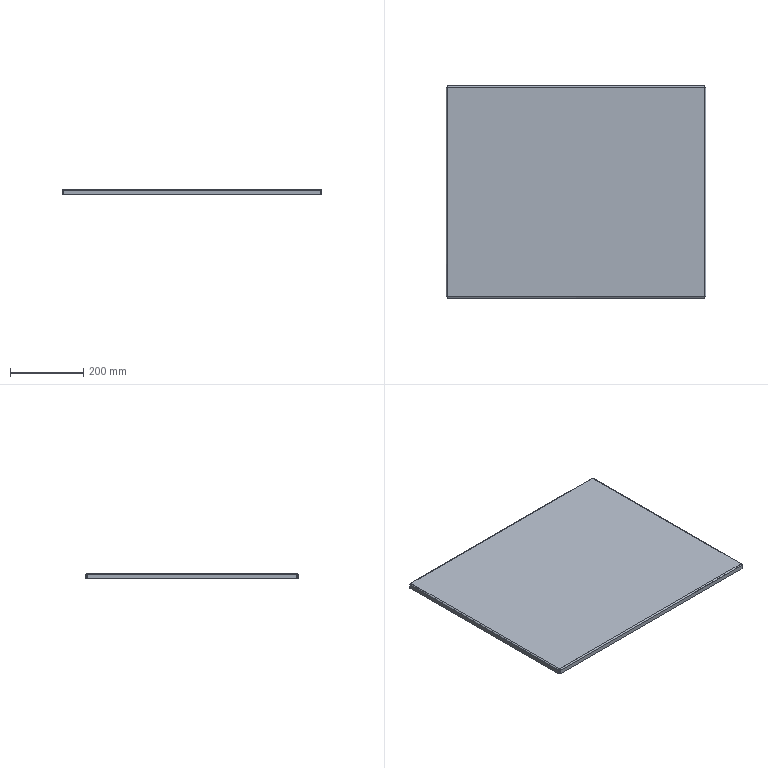Part | STEP file | MYT-A01-P37 | 1 solid | 38 faces | box 710 x 580 x 15 mm | volume 1319701 mm3 | plane 22 | spline 8 | cylinder 8 | commonest cylinder face diameters 1.473 x4 7.473 x4
STEP:
#1=CARTESIAN_POINT('',(-351.263,-286.263,-3.));
#2=VERTEX_POINT('',#1);
#3=CARTESIAN_POINT('',(351.263,-286.263,-3.));
#4=VERTEX_POINT('',#3);
#5=CARTESIAN_POINT('',(-351.293,-286.263,-3.));
#6=DIRECTION('',(1.,0.,0.));
#7=VECTOR('',#6,1000.);
#8=LINE('',#5,#7);
#9=EDGE_CURVE('',#2,#4,#8,.T.);
#10=ORIENTED_EDGE('',*,*,#9,.F.);
#11=CARTESIAN_POINT('',(-351.263,286.263,-3.));
#12=VERTEX_POINT('',#11);
#13=CARTESIAN_POINT('',(-351.263,286.293,-3.));
#14=DIRECTION('',(0.,-1.,0.));
#15=VECTOR('',#14,1000.);
#16=LINE('',#13,#15);
#17=EDGE_CURVE('',#12,#2,#16,.T.);
#18=ORIENTED_EDGE('',*,*,#17,.F.);
#19=CARTESIAN_POINT('',(351.263,286.263,-3.));
#20=VERTEX_POINT('',#19);
#21=CARTESIAN_POINT('',(351.293,286.263,-3.));
#22=DIRECTION('',(-1.,0.,0.));
#23=VECTOR('',#22,1000.);
#24=LINE('',#21,#23);
#25=EDGE_CURVE('',#20,#12,#24,.T.);
#26=ORIENTED_EDGE('',*,*,#25,.F.);
#27=CARTESIAN_POINT('',(351.263,-286.293,-3.));
#28=DIRECTION('',(0.,1.,0.));
#29=VECTOR('',#28,1000.);
#30=LINE('',#27,#29);
#31=EDGE_CURVE('',#4,#20,#30,.T.);
#32=ORIENTED_EDGE('',*,*,#31,.F.);
#33=EDGE_LOOP('',(#10,#18,#26,#32));
#34=FACE_OUTER_BOUND('',#33,.T.);
#35=CARTESIAN_POINT('',(0.,0.,-3.));
#36=DIRECTION('',(0.,0.,1.));
#37=DIRECTION('',(1.,0.,0.));
#38=AXIS2_PLACEMENT_3D('',#35,#36,#37);
#39=PLANE('',#38);
#40=ADVANCED_FACE('',(#34),#39,.F.);
#41=CARTESIAN_POINT('',(-351.263,286.263,0.));
#42=VERTEX_POINT('',#41);
#43=CARTESIAN_POINT('',(-351.263,-286.263,0.));
#44=VERTEX_POINT('',#43);
#45=CARTESIAN_POINT('',(-351.263,286.293,0.));
#46=DIRECTION('',(0.,-1.,0.));
#47=VECTOR('',#46,1000.);
#48=LINE('',#45,#47);
#49=EDGE_CURVE('',#42,#44,#48,.T.);
#50=ORIENTED_EDGE('',*,*,#49,.T.);
#51=CARTESIAN_POINT('',(351.263,-286.263,0.));
#52=VERTEX_POINT('',#51);
#53=CARTESIAN_POINT('',(-351.293,-286.263,0.));
#54=DIRECTION('',(1.,0.,0.));
#55=VECTOR('',#54,1000.);
#56=LINE('',#53,#55);
#57=EDGE_CURVE('',#44,#52,#56,.T.);
#58=ORIENTED_EDGE('',*,*,#57,.T.);
#59=CARTESIAN_POINT('',(351.263,286.263,0.));
#60=VERTEX_POINT('',#59);
#61=CARTESIAN_POINT('',(351.263,-286.293,0.));
#62=DIRECTION('',(0.,1.,0.));
#63=VECTOR('',#62,1000.);
#64=LINE('',#61,#63);
#65=EDGE_CURVE('',#52,#60,#64,.T.);
#66=ORIENTED_EDGE('',*,*,#65,.T.);
#67=CARTESIAN_POINT('',(351.293,286.263,0.));
#68=DIRECTION('',(-1.,0.,0.));
#69=VECTOR('',#68,1000.);
#70=LINE('',#67,#69);
#71=EDGE_CURVE('',#60,#42,#70,.T.);
#72=ORIENTED_EDGE('',*,*,#71,.T.);
#73=EDGE_LOOP('',(#50,#58,#66,#72));
#74=FACE_OUTER_BOUND('',#73,.T.);
#75=CARTESIAN_POINT('',(0.,0.,0.));
#76=DIRECTION('',(0.,0.,1.));
#77=DIRECTION('',(1.,0.,0.));
#78=AXIS2_PLACEMENT_3D('',#75,#76,#77);
#79=PLANE('',#78);
#80=ADVANCED_FACE('',(#74),#79,.T.);
#81=CARTESIAN_POINT('',(355.,286.293,-3.737));
#82=VERTEX_POINT('',#81);
#83=CARTESIAN_POINT('',(352.,286.293,-3.737));
#84=VERTEX_POINT('',#83);
#85=CARTESIAN_POINT('',(352.,286.293,-3.737));
#86=DIRECTION('',(-1.,0.,0.));
#87=VECTOR('',#86,1000.);
#88=LINE('',#85,#87);
#89=EDGE_CURVE('',#82,#84,#88,.T.);
#90=ORIENTED_EDGE('',*,*,#89,.T.);
#91=CARTESIAN_POINT('',(351.263,286.263,-3.));
#92=CARTESIAN_POINT('',(351.456,286.268,-3.));
#93=CARTESIAN_POINT('',(351.648,286.273,-3.079));
#94=CARTESIAN_POINT('',(351.921,286.283,-3.352));
#95=CARTESIAN_POINT('',(352.,286.288,-3.544));
#96=CARTESIAN_POINT('',(352.,286.293,-3.737));
#97=B_SPLINE_CURVE_WITH_KNOTS('',3,(#91,#92,#93,#94,#95,#96),.UNSPECIFIED.,.F.,.F.,(4,2,4),(0.,0.5,1.),.UNSPECIFIED.);
#98=EDGE_CURVE('',#20,#84,#97,.T.);
#99=ORIENTED_EDGE('',*,*,#98,.F.);
#100=CARTESIAN_POINT('',(351.263,286.263,-3.));
#101=DIRECTION('',(0.,0.,1.));
#102=VECTOR('',#101,1000.);
#103=LINE('',#100,#102);
#104=EDGE_CURVE('',#20,#60,#103,.T.);
#105=ORIENTED_EDGE('',*,*,#104,.T.);
#106=CARTESIAN_POINT('',(351.263,286.263,0.));
#107=CARTESIAN_POINT('',(351.753,286.266,0.));
#108=CARTESIAN_POINT('',(352.241,286.268,-0.09725));
#109=CARTESIAN_POINT('',(353.145,286.273,-0.4716));
#110=CARTESIAN_POINT('',(353.56,286.276,-0.7486));
#111=CARTESIAN_POINT('',(354.251,286.281,-1.44));
#112=CARTESIAN_POINT('',(354.528,286.283,-1.855));
#113=CARTESIAN_POINT('',(354.903,286.288,-2.759));
#114=CARTESIAN_POINT('',(355.,286.29,-3.247));
#115=CARTESIAN_POINT('',(355.,286.293,-3.737));
#116=B_SPLINE_CURVE_WITH_KNOTS('',3,(#106,#107,#108,#109,#110,#111,#112,#113,#114,#115),.UNSPECIFIED.,.F.,.F.,(4,2,2,2,4),(0.,0.25,0.5,0.75,1.),.UNSPECIFIED.);
#117=EDGE_CURVE('',#60,#82,#116,.T.);
#118=ORIENTED_EDGE('',*,*,#117,.T.);
#119=EDGE_LOOP('',(#90,#99,#105,#118));
#120=FACE_OUTER_BOUND('',#119,.T.);
#121=CARTESIAN_POINT('',(351.263,286.263,0.03));
#122=CARTESIAN_POINT('',(351.757,286.266,0.03));
#123=CARTESIAN_POINT('',(352.249,286.268,-0.06803));
#124=CARTESIAN_POINT('',(353.16,286.273,-0.4454));
#125=CARTESIAN_POINT('',(353.578,286.276,-0.7246));
#126=CARTESIAN_POINT('',(354.275,286.281,-1.422));
#127=CARTESIAN_POINT('',(354.555,286.283,-1.84));
#128=CARTESIAN_POINT('',(354.932,286.288,-2.751));
#129=CARTESIAN_POINT('',(355.03,286.29,-3.243));
#130=CARTESIAN_POINT('',(355.03,286.293,-3.737));
#131=CARTESIAN_POINT('',(351.263,286.263,0.));
#132=CARTESIAN_POINT('',(351.753,286.266,0.));
#133=CARTESIAN_POINT('',(352.241,286.268,-0.09725));
#134=CARTESIAN_POINT('',(353.145,286.273,-0.4716));
#135=CARTESIAN_POINT('',(353.56,286.276,-0.7486));
#136=CARTESIAN_POINT('',(354.251,286.281,-1.44));
#137=CARTESIAN_POINT('',(354.528,286.283,-1.855));
#138=CARTESIAN_POINT('',(354.903,286.288,-2.759));
#139=CARTESIAN_POINT('',(355.,286.29,-3.247));
#140=CARTESIAN_POINT('',(355.,286.293,-3.737));
#141=CARTESIAN_POINT('',(351.263,286.263,-3.));
#142=CARTESIAN_POINT('',(351.36,286.266,-3.));
#143=CARTESIAN_POINT('',(351.456,286.268,-3.019));
#144=CARTESIAN_POINT('',(351.634,286.273,-3.093));
#145=CARTESIAN_POINT('',(351.716,286.276,-3.148));
#146=CARTESIAN_POINT('',(351.852,286.281,-3.284));
#147=CARTESIAN_POINT('',(351.907,286.283,-3.366));
#148=CARTESIAN_POINT('',(351.981,286.288,-3.544));
#149=CARTESIAN_POINT('',(352.,286.29,-3.64));
#150=CARTESIAN_POINT('',(352.,286.293,-3.737));
#151=CARTESIAN_POINT('',(351.263,286.263,-3.03));
#152=CARTESIAN_POINT('',(351.356,286.266,-3.03));
#153=CARTESIAN_POINT('',(351.448,286.268,-3.049));
#154=CARTESIAN_POINT('',(351.619,286.273,-3.119));
#155=CARTESIAN_POINT('',(351.697,286.276,-3.172));
#156=CARTESIAN_POINT('',(351.828,286.281,-3.303));
#157=CARTESIAN_POINT('',(351.881,286.283,-3.381));
#158=CARTESIAN_POINT('',(351.951,286.288,-3.552));
#159=CARTESIAN_POINT('',(351.97,286.29,-3.644));
#160=CARTESIAN_POINT('',(351.97,286.293,-3.737));
#161=B_SPLINE_SURFACE_WITH_KNOTS('',1,3,((#121,#122,#123,#124,#125,#126,#127,#128,#129,#130),(#131,#132,#133,#134,#135,#136,#137,#138,#139,#140),(#141,#142,#143,#144,#145,#146,#147,#148,#149,#150),(#151,#152,#153,#154,#155,#156,#157,#158,#159,#160)),.UNSPECIFIED.,.F.,.F.,.F.,(2,1,1,2),(4,2,2,2,4),(-0.01,0.,1.,1.01),(0.,0.25,0.5,0.75,1.),.UNSPECIFIED.);
#162=ADVANCED_FACE('',(#120),#161,.F.);
#163=CARTESIAN_POINT('',(352.,-286.293,-3.737));
#164=VERTEX_POINT('',#163);
#165=CARTESIAN_POINT('',(352.,-286.293,-3.737));
#166=CARTESIAN_POINT('',(352.,-286.288,-3.544));
#167=CARTESIAN_POINT('',(351.921,-286.283,-3.352));
#168=CARTESIAN_POINT('',(351.648,-286.273,-3.079));
#169=CARTESIAN_POINT('',(351.456,-286.268,-3.));
#170=CARTESIAN_POINT('',(351.263,-286.263,-3.));
#171=B_SPLINE_CURVE_WITH_KNOTS('',3,(#165,#166,#167,#168,#169,#170),.UNSPECIFIED.,.F.,.F.,(4,2,4),(0.,0.5,1.),.UNSPECIFIED.);
#172=EDGE_CURVE('',#164,#4,#171,.T.);
#173=ORIENTED_EDGE('',*,*,#172,.F.);
#174=CARTESIAN_POINT('',(355.,-286.293,-3.737));
#175=VERTEX_POINT('',#174);
#176=CARTESIAN_POINT('',(352.,-286.293,-3.737));
#177=DIRECTION('',(-1.,0.,0.));
#178=VECTOR('',#177,1000.);
#179=LINE('',#176,#178);
#180=EDGE_CURVE('',#175,#164,#179,.T.);
#181=ORIENTED_EDGE('',*,*,#180,.F.);
#182=CARTESIAN_POINT('',(355.,-286.293,-3.737));
#183=CARTESIAN_POINT('',(355.,-286.29,-3.247));
#184=CARTESIAN_POINT('',(354.903,-286.288,-2.759));
#185=CARTESIAN_POINT('',(354.528,-286.283,-1.855));
#186=CARTESIAN_POINT('',(354.251,-286.281,-1.44));
#187=CARTESIAN_POINT('',(353.56,-286.276,-0.7486));
#188=CARTESIAN_POINT('',(353.145,-286.273,-0.4716));
#189=CARTESIAN_POINT('',(352.241,-286.268,-0.09725));
#190=CARTESIAN_POINT('',(351.753,-286.266,0.));
#191=CARTESIAN_POINT('',(351.263,-286.263,0.));
#192=B_SPLINE_CURVE_WITH_KNOTS('',3,(#182,#183,#184,#185,#186,#187,#188,#189,#190,#191),.UNSPECIFIED.,.F.,.F.,(4,2,2,2,4),(0.,0.25,0.5,0.75,1.),.UNSPECIFIED.);
#193=EDGE_CURVE('',#175,#52,#192,.T.);
#194=ORIENTED_EDGE('',*,*,#193,.T.);
#195=CARTESIAN_POINT('',(351.263,-286.263,-3.));
#196=DIRECTION('',(0.,0.,1.));
#197=VECTOR('',#196,1000.);
#198=LINE('',#195,#197);
#199=EDGE_CURVE('',#4,#52,#198,.T.);
#200=ORIENTED_EDGE('',*,*,#199,.F.);
#201=EDGE_LOOP('',(#173,#181,#194,#200));
#202=FACE_OUTER_BOUND('',#201,.T.);
#203=CARTESIAN_POINT('',(355.03,-286.293,-3.737));
#204=CARTESIAN_POINT('',(355.03,-286.29,-3.243));
#205=CARTESIAN_POINT('',(354.932,-286.288,-2.751));
#206=CARTESIAN_POINT('',(354.555,-286.283,-1.84));
#207=CARTESIAN_POINT('',(354.275,-286.281,-1.422));
#208=CARTESIAN_POINT('',(353.578,-286.276,-0.7246));
#209=CARTESIAN_POINT('',(353.16,-286.273,-0.4454));
#210=CARTESIAN_POINT('',(352.249,-286.268,-0.06803));
#211=CARTESIAN_POINT('',(351.757,-286.266,0.03));
#212=CARTESIAN_POINT('',(351.263,-286.263,0.03));
#213=CARTESIAN_POINT('',(355.,-286.293,-3.737));
#214=CARTESIAN_POINT('',(355.,-286.29,-3.247));
#215=CARTESIAN_POINT('',(354.903,-286.288,-2.759));
#216=CARTESIAN_POINT('',(354.528,-286.283,-1.855));
#217=CARTESIAN_POINT('',(354.251,-286.281,-1.44));
#218=CARTESIAN_POINT('',(353.56,-286.276,-0.7486));
#219=CARTESIAN_POINT('',(353.145,-286.273,-0.4716));
#220=CARTESIAN_POINT('',(352.241,-286.268,-0.09725));
#221=CARTESIAN_POINT('',(351.753,-286.266,0.));
#222=CARTESIAN_POINT('',(351.263,-286.263,0.));
#223=CARTESIAN_POINT('',(352.,-286.293,-3.737));
#224=CARTESIAN_POINT('',(352.,-286.29,-3.64));
#225=CARTESIAN_POINT('',(351.981,-286.288,-3.544));
#226=CARTESIAN_POINT('',(351.907,-286.283,-3.366));
#227=CARTESIAN_POINT('',(351.852,-286.281,-3.284));
#228=CARTESIAN_POINT('',(351.716,-286.276,-3.148));
#229=CARTESIAN_POINT('',(351.634,-286.273,-3.093));
#230=CARTESIAN_POINT('',(351.456,-286.268,-3.019));
#231=CARTESIAN_POINT('',(351.36,-286.266,-3.));
#232=CARTESIAN_POINT('',(351.263,-286.263,-3.));
#233=CARTESIAN_POINT('',(351.97,-286.293,-3.737));
#234=CARTESIAN_POINT('',(351.97,-286.29,-3.644));
#235=CARTESIAN_POINT('',(351.951,-286.288,-3.552));
#236=CARTESIAN_POINT('',(351.881,-286.283,-3.381));
#237=CARTESIAN_POINT('',(351.828,-286.281,-3.303));
#238=CARTESIAN_POINT('',(351.697,-286.276,-3.172));
#239=CARTESIAN_POINT('',(351.619,-286.273,-3.119));
#240=CARTESIAN_POINT('',(351.448,-286.268,-3.049));
#241=CARTESIAN_POINT('',(351.356,-286.266,-3.03));
#242=CARTESIAN_POINT('',(351.263,-286.263,-3.03));
#243=B_SPLINE_SURFACE_WITH_KNOTS('',1,3,((#203,#204,#205,#206,#207,#208,#209,#210,#211,#212),(#213,#214,#215,#216,#217,#218,#219,#220,#221,#222),(#223,#224,#225,#226,#227,#228,#229,#230,#231,#232),(#233,#234,#235,#236,#237,#238,#239,#240,#241,#242)),.UNSPECIFIED.,.F.,.F.,.F.,(2,1,1,2),(4,2,2,2,4),(-0.01,0.,1.,1.01),(0.,0.25,0.5,0.75,1.),.UNSPECIFIED.);
#244=ADVANCED_FACE('',(#202),#243,.F.);
#245=ORIENTED_EDGE('',*,*,#65,.F.);
#246=ORIENTED_EDGE('',*,*,#193,.F.);
#247=CARTESIAN_POINT('',(355.,290.,-3.737));
#248=DIRECTION('',(0.,1.,0.));
#249=VECTOR('',#248,1000.);
#250=LINE('',#247,#249);
#251=EDGE_CURVE('',#175,#82,#250,.T.);
#252=ORIENTED_EDGE('',*,*,#251,.T.);
#253=ORIENTED_EDGE('',*,*,#117,.F.);
#254=EDGE_LOOP('',(#245,#246,#252,#253));
#255=FACE_OUTER_BOUND('',#254,.T.);
#256=CARTESIAN_POINT('',(351.263,-286.293,-3.737));
#257=DIRECTION('',(0.,-1.,0.));
#258=DIRECTION('',(1.,0.,0.));
#259=AXIS2_PLACEMENT_3D('',#256,#257,#258);
#260=CYLINDRICAL_SURFACE('',#259,3.737);
#261=ADVANCED_FACE('',(#255),#260,.T.);
#262=ORIENTED_EDGE('',*,*,#31,.T.);
#263=ORIENTED_EDGE('',*,*,#98,.T.);
#264=CARTESIAN_POINT('',(352.,290.,-3.737));
#265=DIRECTION('',(0.,-1.,0.));
#266=VECTOR('',#265,1000.);
#267=LINE('',#264,#266);
#268=EDGE_CURVE('',#84,#164,#267,.T.);
#269=ORIENTED_EDGE('',*,*,#268,.T.);
#270=ORIENTED_EDGE('',*,*,#172,.T.);
#271=EDGE_LOOP('',(#262,#263,#269,#270));
#272=FACE_OUTER_BOUND('',#271,.T.);
#273=CARTESIAN_POINT('',(351.263,-286.293,-3.737));
#274=DIRECTION('',(0.,-1.,0.));
#275=DIRECTION('',(1.,0.,0.));
#276=AXIS2_PLACEMENT_3D('',#273,#274,#275);
#277=CYLINDRICAL_SURFACE('',#276,0.7366);
#278=ADVANCED_FACE('',(#272),#277,.F.);
#279=CARTESIAN_POINT('',(355.,286.293,-15.));
#280=VERTEX_POINT('',#279);
#281=CARTESIAN_POINT('',(355.,286.293,-3.));
#282=DIRECTION('',(0.,0.,-1.));
#283=VECTOR('',#282,1000.);
#284=LINE('',#281,#283);
#285=EDGE_CURVE('',#82,#280,#284,.T.);
#286=ORIENTED_EDGE('',*,*,#285,.T.);
#287=CARTESIAN_POINT('',(352.,286.293,-15.));
#288=VERTEX_POINT('',#287);
#289=CARTESIAN_POINT('',(352.,286.293,-15.));
#290=DIRECTION('',(-1.,0.,0.));
#291=VECTOR('',#290,1000.);
#292=LINE('',#289,#291);
#293=EDGE_CURVE('',#280,#288,#292,.T.);
#294=ORIENTED_EDGE('',*,*,#293,.T.);
#295=CARTESIAN_POINT('',(352.,286.293,0.));
#296=DIRECTION('',(0.,0.,-1.));
#297=VECTOR('',#296,1000.);
#298=LINE('',#295,#297);
#299=EDGE_CURVE('',#84,#288,#298,.T.);
#300=ORIENTED_EDGE('',*,*,#299,.F.);
#301=ORIENTED_EDGE('',*,*,#89,.F.);
#302=EDGE_LOOP('',(#286,#294,#300,#301));
#303=FACE_OUTER_BOUND('',#302,.T.);
#304=CARTESIAN_POINT('',(352.,286.293,-3.));
#305=DIRECTION('',(0.,1.,0.));
#306=DIRECTION('',(0.,0.,1.));
#307=AXIS2_PLACEMENT_3D('',#304,#305,#306);
#308=PLANE('',#307);
#309=ADVANCED_FACE('',(#303),#308,.T.);
#310=ORIENTED_EDGE('',*,*,#285,.F.);
#311=ORIENTED_EDGE('',*,*,#251,.F.);
#312=CARTESIAN_POINT('',(355.,-286.293,-15.));
#313=VERTEX_POINT('',#312);
#314=CARTESIAN_POINT('',(355.,-286.293,0.));
#315=DIRECTION('',(0.,0.,-1.));
#316=VECTOR('',#315,1000.);
#317=LINE('',#314,#316);
#318=EDGE_CURVE('',#175,#313,#317,.T.);
#319=ORIENTED_EDGE('',*,*,#318,.T.);
#320=CARTESIAN_POINT('',(355.,0.,-15.));
#321=DIRECTION('',(0.,1.,0.));
#322=VECTOR('',#321,1000.);
#323=LINE('',#320,#322);
#324=EDGE_CURVE('',#313,#280,#323,.T.);
#325=ORIENTED_EDGE('',*,*,#324,.T.);
#326=EDGE_LOOP('',(#310,#311,#319,#325));
#327=FACE_OUTER_BOUND('',#326,.T.);
#328=CARTESIAN_POINT('',(355.,0.,0.));
#329=DIRECTION('',(-1.,0.,0.));
#330=DIRECTION('',(0.,-1.,0.));
#331=AXIS2_PLACEMENT_3D('',#328,#329,#330);
#332=PLANE('',#331);
#333=ADVANCED_FACE('',(#327),#332,.F.);
#334=ORIENTED_EDGE('',*,*,#268,.F.);
#335=ORIENTED_EDGE('',*,*,#299,.T.);
#336=CARTESIAN_POINT('',(352.,-286.293,-15.));
#337=VERTEX_POINT('',#336);
#338=CARTESIAN_POINT('',(352.,290.,-15.));
#339=DIRECTION('',(0.,1.,0.));
#340=VECTOR('',#339,1000.);
#341=LINE('',#338,#340);
#342=EDGE_CURVE('',#337,#288,#341,.T.);
#343=ORIENTED_EDGE('',*,*,#342,.F.);
#344=CARTESIAN_POINT('',(352.,-286.293,-3.));
#345=DIRECTION('',(0.,0.,-1.));
#346=VECTOR('',#345,1000.);
#347=LINE('',#344,#346);
#348=EDGE_CURVE('',#164,#337,#347,.T.);
#349=ORIENTED_EDGE('',*,*,#348,.F.);
#350=EDGE_LOOP('',(#334,#335,#343,#349));
#351=FACE_OUTER_BOUND('',#350,.T.);
#352=CARTESIAN_POINT('',(352.,0.,0.));
#353=DIRECTION('',(-1.,0.,0.));
#354=DIRECTION('',(0.,-1.,0.));
#355=AXIS2_PLACEMENT_3D('',#352,#353,#354);
#356=PLANE('',#355);
#357=ADVANCED_FACE('',(#351),#356,.T.);
#358=ORIENTED_EDGE('',*,*,#293,.F.);
#359=ORIENTED_EDGE('',*,*,#324,.F.);
#360=CARTESIAN_POINT('',(355.,-286.293,-15.));
#361=DIRECTION('',(-1.,0.,0.));
#362=VECTOR('',#361,1000.);
#363=LINE('',#360,#362);
#364=EDGE_CURVE('',#313,#337,#363,.T.);
#365=ORIENTED_EDGE('',*,*,#364,.T.);
#366=ORIENTED_EDGE('',*,*,#342,.T.);
#367=EDGE_LOOP('',(#358,#359,#365,#366));
#368=FACE_OUTER_BOUND('',#367,.T.);
#369=CARTESIAN_POINT('',(355.,290.,-15.));
#370=DIRECTION('',(0.,0.,1.));
#371=DIRECTION('',(1.,0.,0.));
#372=AXIS2_PLACEMENT_3D('',#369,#370,#371);
#373=PLANE('',#372);
#374=ADVANCED_FACE('',(#368),#373,.F.);
#375=ORIENTED_EDGE('',*,*,#364,.F.);
#376=ORIENTED_EDGE('',*,*,#318,.F.);
#377=ORIENTED_EDGE('',*,*,#180,.T.);
#378=ORIENTED_EDGE('',*,*,#348,.T.);
#379=EDGE_LOOP('',(#375,#376,#377,#378));
#380=FACE_OUTER_BOUND('',#379,.T.);
#381=CARTESIAN_POINT('',(352.,-286.293,-3.));
#382=DIRECTION('',(0.,1.,0.));
#383=DIRECTION('',(0.,0.,1.));
#384=AXIS2_PLACEMENT_3D('',#381,#382,#383);
#385=PLANE('',#384);
#386=ADVANCED_FACE('',(#380),#385,.F.);
#387=CARTESIAN_POINT('',(-351.293,290.,-3.737));
#388=VERTEX_POINT('',#387);
#389=CARTESIAN_POINT('',(-351.293,287.,-3.737));
#390=VERTEX_POINT('',#389);
#391=CARTESIAN_POINT('',(-351.293,287.,-3.737));
#392=DIRECTION('',(0.,-1.,0.));
#393=VECTOR('',#392,1000.);
#394=LINE('',#391,#393);
#395=EDGE_CURVE('',#388,#390,#394,.T.);
#396=ORIENTED_EDGE('',*,*,#395,.T.);
#397=CARTESIAN_POINT('',(-351.263,286.263,-3.));
#398=CARTESIAN_POINT('',(-351.268,286.456,-3.));
#399=CARTESIAN_POINT('',(-351.273,286.648,-3.079));
#400=CARTESIAN_POINT('',(-351.283,286.921,-3.352));
#401=CARTESIAN_POINT('',(-351.288,287.,-3.544));
#402=CARTESIAN_POINT('',(-351.293,287.,-3.737));
#403=B_SPLINE_CURVE_WITH_KNOTS('',3,(#397,#398,#399,#400,#401,#402),.UNSPECIFIED.,.F.,.F.,(4,2,4),(0.,0.5,1.),.UNSPECIFIED.);
#404=EDGE_CURVE('',#12,#390,#403,.T.);
#405=ORIENTED_EDGE('',*,*,#404,.F.);
#406=CARTESIAN_POINT('',(-351.263,286.263,-3.));
#407=DIRECTION('',(0.,0.,1.));
#408=VECTOR('',#407,1000.);
#409=LINE('',#406,#408);
#410=EDGE_CURVE('',#12,#42,#409,.T.);
#411=ORIENTED_EDGE('',*,*,#410,.T.);
#412=CARTESIAN_POINT('',(-351.263,286.263,0.));
#413=CARTESIAN_POINT('',(-351.266,286.753,0.));
#414=CARTESIAN_POINT('',(-351.268,287.241,-0.09725));
#415=CARTESIAN_POINT('',(-351.273,288.145,-0.4716));
#416=CARTESIAN_POINT('',(-351.276,288.56,-0.7486));
#417=CARTESIAN_POINT('',(-351.281,289.251,-1.44));
#418=CARTESIAN_POINT('',(-351.283,289.528,-1.855));
#419=CARTESIAN_POINT('',(-351.288,289.903,-2.759));
#420=CARTESIAN_POINT('',(-351.29,290.,-3.247));
#421=CARTESIAN_POINT('',(-351.293,290.,-3.737));
#422=B_SPLINE_CURVE_WITH_KNOTS('',3,(#412,#413,#414,#415,#416,#417,#418,#419,#420,#421),.UNSPECIFIED.,.F.,.F.,(4,2,2,2,4),(0.,0.25,0.5,0.75,1.),.UNSPECIFIED.);
#423=EDGE_CURVE('',#42,#388,#422,.T.);
#424=ORIENTED_EDGE('',*,*,#423,.T.);
#425=EDGE_LOOP('',(#396,#405,#411,#424));
#426=FACE_OUTER_BOUND('',#425,.T.);
#427=CARTESIAN_POINT('',(-351.263,286.263,0.03));
#428=CARTESIAN_POINT('',(-351.266,286.757,0.03));
#429=CARTESIAN_POINT('',(-351.268,287.249,-0.06803));
#430=CARTESIAN_POINT('',(-351.273,288.16,-0.4454));
#431=CARTESIAN_POINT('',(-351.276,288.578,-0.7246));
#432=CARTESIAN_POINT('',(-351.281,289.275,-1.422));
#433=CARTESIAN_POINT('',(-351.283,289.555,-1.84));
#434=CARTESIAN_POINT('',(-351.288,289.932,-2.751));
#435=CARTESIAN_POINT('',(-351.29,290.03,-3.243));
#436=CARTESIAN_POINT('',(-351.293,290.03,-3.737));
#437=CARTESIAN_POINT('',(-351.263,286.263,0.));
#438=CARTESIAN_POINT('',(-351.266,286.753,0.));
#439=CARTESIAN_POINT('',(-351.268,287.241,-0.09725));
#440=CARTESIAN_POINT('',(-351.273,288.145,-0.4716));
#441=CARTESIAN_POINT('',(-351.276,288.56,-0.7486));
#442=CARTESIAN_POINT('',(-351.281,289.251,-1.44));
#443=CARTESIAN_POINT('',(-351.283,289.528,-1.855));
#444=CARTESIAN_POINT('',(-351.288,289.903,-2.759));
#445=CARTESIAN_POINT('',(-351.29,290.,-3.247));
#446=CARTESIAN_POINT('',(-351.293,290.,-3.737));
#447=CARTESIAN_POINT('',(-351.263,286.263,-3.));
#448=CARTESIAN_POINT('',(-351.266,286.36,-3.));
#449=CARTESIAN_POINT('',(-351.268,286.456,-3.019));
#450=CARTESIAN_POINT('',(-351.273,286.634,-3.093));
#451=CARTESIAN_POINT('',(-351.276,286.716,-3.148));
#452=CARTESIAN_POINT('',(-351.281,286.852,-3.284));
#453=CARTESIAN_POINT('',(-351.283,286.907,-3.366));
#454=CARTESIAN_POINT('',(-351.288,286.981,-3.544));
#455=CARTESIAN_POINT('',(-351.29,287.,-3.64));
#456=CARTESIAN_POINT('',(-351.293,287.,-3.737));
#457=CARTESIAN_POINT('',(-351.263,286.263,-3.03));
#458=CARTESIAN_POINT('',(-351.266,286.356,-3.03));
#459=CARTESIAN_POINT('',(-351.268,286.448,-3.049));
#460=CARTESIAN_POINT('',(-351.273,286.619,-3.119));
#461=CARTESIAN_POINT('',(-351.276,286.697,-3.172));
#462=CARTESIAN_POINT('',(-351.281,286.828,-3.303));
#463=CARTESIAN_POINT('',(-351.283,286.881,-3.381));
#464=CARTESIAN_POINT('',(-351.288,286.951,-3.552));
#465=CARTESIAN_POINT('',(-351.29,286.97,-3.644));
#466=CARTESIAN_POINT('',(-351.293,286.97,-3.737));
#467=B_SPLINE_SURFACE_WITH_KNOTS('',1,3,((#427,#428,#429,#430,#431,#432,#433,#434,#435,#436),(#437,#438,#439,#440,#441,#442,#443,#444,#445,#446),(#447,#448,#449,#450,#451,#452,#453,#454,#455,#456),(#457,#458,#459,#460,#461,#462,#463,#464,#465,#466)),.UNSPECIFIED.,.F.,.F.,.F.,(2,1,1,2),(4,2,2,2,4),(-0.01,0.,1.,1.01),(0.,0.25,0.5,0.75,1.),.UNSPECIFIED.);
#468=ADVANCED_FACE('',(#426),#467,.F.);
#469=CARTESIAN_POINT('',(351.293,287.,-3.737));
#470=VERTEX_POINT('',#469);
#471=CARTESIAN_POINT('',(351.293,287.,-3.737));
#472=CARTESIAN_POINT('',(351.288,287.,-3.544));
#473=CARTESIAN_POINT('',(351.283,286.921,-3.352));
#474=CARTESIAN_POINT('',(351.273,286.648,-3.079));
#475=CARTESIAN_POINT('',(351.268,286.456,-3.));
#476=CARTESIAN_POINT('',(351.263,286.263,-3.));
#477=B_SPLINE_CURVE_WITH_KNOTS('',3,(#471,#472,#473,#474,#475,#476),.UNSPECIFIED.,.F.,.F.,(4,2,4),(0.,0.5,1.),.UNSPECIFIED.);
#478=EDGE_CURVE('',#470,#20,#477,.T.);
#479=ORIENTED_EDGE('',*,*,#478,.F.);
#480=CARTESIAN_POINT('',(351.293,290.,-3.737));
#481=VERTEX_POINT('',#480);
#482=CARTESIAN_POINT('',(351.293,287.,-3.737));
#483=DIRECTION('',(0.,-1.,0.));
#484=VECTOR('',#483,1000.);
#485=LINE('',#482,#484);
#486=EDGE_CURVE('',#481,#470,#485,.T.);
#487=ORIENTED_EDGE('',*,*,#486,.F.);
#488=CARTESIAN_POINT('',(351.293,290.,-3.737));
#489=CARTESIAN_POINT('',(351.29,290.,-3.247));
#490=CARTESIAN_POINT('',(351.288,289.903,-2.759));
#491=CARTESIAN_POINT('',(351.283,289.528,-1.855));
#492=CARTESIAN_POINT('',(351.281,289.251,-1.44));
#493=CARTESIAN_POINT('',(351.276,288.56,-0.7486));
#494=CARTESIAN_POINT('',(351.273,288.145,-0.4716));
#495=CARTESIAN_POINT('',(351.268,287.241,-0.09725));
#496=CARTESIAN_POINT('',(351.266,286.753,0.));
#497=CARTESIAN_POINT('',(351.263,286.263,0.));
#498=B_SPLINE_CURVE_WITH_KNOTS('',3,(#488,#489,#490,#491,#492,#493,#494,#495,#496,#497),.UNSPECIFIED.,.F.,.F.,(4,2,2,2,4),(0.,0.25,0.5,0.75,1.),.UNSPECIFIED.);
#499=EDGE_CURVE('',#481,#60,#498,.T.);
#500=ORIENTED_EDGE('',*,*,#499,.T.);
#501=ORIENTED_EDGE('',*,*,#104,.F.);
#502=EDGE_LOOP('',(#479,#487,#500,#501));
#503=FACE_OUTER_BOUND('',#502,.T.);
#504=CARTESIAN_POINT('',(351.293,290.03,-3.737));
#505=CARTESIAN_POINT('',(351.29,290.03,-3.243));
#506=CARTESIAN_POINT('',(351.288,289.932,-2.751));
#507=CARTESIAN_POINT('',(351.283,289.555,-1.84));
#508=CARTESIAN_POINT('',(351.281,289.275,-1.422));
#509=CARTESIAN_POINT('',(351.276,288.578,-0.7246));
#510=CARTESIAN_POINT('',(351.273,288.16,-0.4454));
#511=CARTESIAN_POINT('',(351.268,287.249,-0.06803));
#512=CARTESIAN_POINT('',(351.266,286.757,0.03));
#513=CARTESIAN_POINT('',(351.263,286.263,0.03));
#514=CARTESIAN_POINT('',(351.293,290.,-3.737));
#515=CARTESIAN_POINT('',(351.29,290.,-3.247));
#516=CARTESIAN_POINT('',(351.288,289.903,-2.759));
#517=CARTESIAN_POINT('',(351.283,289.528,-1.855));
#518=CARTESIAN_POINT('',(351.281,289.251,-1.44));
#519=CARTESIAN_POINT('',(351.276,288.56,-0.7486));
#520=CARTESIAN_POINT('',(351.273,288.145,-0.4716));
#521=CARTESIAN_POINT('',(351.268,287.241,-0.09725));
#522=CARTESIAN_POINT('',(351.266,286.753,0.));
#523=CARTESIAN_POINT('',(351.263,286.263,0.));
#524=CARTESIAN_POINT('',(351.293,287.,-3.737));
#525=CARTESIAN_POINT('',(351.29,287.,-3.64));
#526=CARTESIAN_POINT('',(351.288,286.981,-3.544));
#527=CARTESIAN_POINT('',(351.283,286.907,-3.366));
#528=CARTESIAN_POINT('',(351.281,286.852,-3.284));
#529=CARTESIAN_POINT('',(351.276,286.716,-3.148));
#530=CARTESIAN_POINT('',(351.273,286.634,-3.093));
#531=CARTESIAN_POINT('',(351.268,286.456,-3.019));
#532=CARTESIAN_POINT('',(351.266,286.36,-3.));
#533=CARTESIAN_POINT('',(351.263,286.263,-3.));
#534=CARTESIAN_POINT('',(351.293,286.97,-3.737));
#535=CARTESIAN_POINT('',(351.29,286.97,-3.644));
#536=CARTESIAN_POINT('',(351.288,286.951,-3.552));
#537=CARTESIAN_POINT('',(351.283,286.881,-3.381));
#538=CARTESIAN_POINT('',(351.281,286.828,-3.303));
#539=CARTESIAN_POINT('',(351.276,286.697,-3.172));
#540=CARTESIAN_POINT('',(351.273,286.619,-3.119));
#541=CARTESIAN_POINT('',(351.268,286.448,-3.049));
#542=CARTESIAN_POINT('',(351.266,286.356,-3.03));
#543=CARTESIAN_POINT('',(351.263,286.263,-3.03));
#544=B_SPLINE_SURFACE_WITH_KNOTS('',1,3,((#504,#505,#506,#507,#508,#509,#510,#511,#512,#513),(#514,#515,#516,#517,#518,#519,#520,#521,#522,#523),(#524,#525,#526,#527,#528,#529,#530,#531,#532,#533),(#534,#535,#536,#537,#538,#539,#540,#541,#542,#543)),.UNSPECIFIED.,.F.,.F.,.F.,(2,1,1,2),(4,2,2,2,4),(-0.01,0.,1.,1.01),(0.,0.25,0.5,0.75,1.),.UNSPECIFIED.);
#545=ADVANCED_FACE('',(#503),#544,.F.);
#546=ORIENTED_EDGE('',*,*,#71,.F.);
#547=ORIENTED_EDGE('',*,*,#499,.F.);
#548=CARTESIAN_POINT('',(-355.,290.,-3.737));
#549=DIRECTION('',(-1.,0.,0.));
#550=VECTOR('',#549,1000.);
#551=LINE('',#548,#550);
#552=EDGE_CURVE('',#481,#388,#551,.T.);
#553=ORIENTED_EDGE('',*,*,#552,.T.);
#554=ORIENTED_EDGE('',*,*,#423,.F.);
#555=EDGE_LOOP('',(#546,#547,#553,#554));
#556=FACE_OUTER_BOUND('',#555,.T.);
#557=CARTESIAN_POINT('',(351.293,286.263,-3.737));
#558=DIRECTION('',(1.,0.,0.));
#559=DIRECTION('',(0.,1.,0.));
#560=AXIS2_PLACEMENT_3D('',#557,#558,#559);
#561=CYLINDRICAL_SURFACE('',#560,3.737);
#562=ADVANCED_FACE('',(#556),#561,.T.);
#563=ORIENTED_EDGE('',*,*,#25,.T.);
#564=ORIENTED_EDGE('',*,*,#404,.T.);
#565=CARTESIAN_POINT('',(-355.,287.,-3.737));
#566=DIRECTION('',(1.,0.,0.));
#567=VECTOR('',#566,1000.);
#568=LINE('',#565,#567);
#569=EDGE_CURVE('',#390,#470,#568,.T.);
#570=ORIENTED_EDGE('',*,*,#569,.T.);
#571=ORIENTED_EDGE('',*,*,#478,.T.);
#572=EDGE_LOOP('',(#563,#564,#570,#571));
#573=FACE_OUTER_BOUND('',#572,.T.);
#574=CARTESIAN_POINT('',(351.293,286.263,-3.737));
#575=DIRECTION('',(1.,0.,0.));
#576=DIRECTION('',(0.,1.,0.));
#577=AXIS2_PLACEMENT_3D('',#574,#575,#576);
#578=CYLINDRICAL_SURFACE('',#577,0.7366);
#579=ADVANCED_FACE('',(#573),#578,.F.);
#580=CARTESIAN_POINT('',(-351.293,290.,-15.));
#581=VERTEX_POINT('',#580);
#582=CARTESIAN_POINT('',(-351.293,290.,-3.));
#583=DIRECTION('',(0.,0.,-1.));
#584=VECTOR('',#583,1000.);
#585=LINE('',#582,#584);
#586=EDGE_CURVE('',#388,#581,#585,.T.);
#587=ORIENTED_EDGE('',*,*,#586,.T.);
#588=CARTESIAN_POINT('',(-351.293,287.,-15.));
#589=VERTEX_POINT('',#588);
#590=CARTESIAN_POINT('',(-351.293,287.,-15.));
#591=DIRECTION('',(0.,-1.,0.));
#592=VECTOR('',#591,1000.);
#593=LINE('',#590,#592);
#594=EDGE_CURVE('',#581,#589,#593,.T.);
#595=ORIENTED_EDGE('',*,*,#594,.T.);
#596=CARTESIAN_POINT('',(-351.293,287.,0.));
#597=DIRECTION('',(0.,0.,-1.));
#598=VECTOR('',#597,1000.);
#599=LINE('',#596,#598);
#600=EDGE_CURVE('',#390,#589,#599,.T.);
#601=ORIENTED_EDGE('',*,*,#600,.F.);
#602=ORIENTED_EDGE('',*,*,#395,.F.);
#603=EDGE_LOOP('',(#587,#595,#601,#602));
#604=FACE_OUTER_BOUND('',#603,.T.);
#605=CARTESIAN_POINT('',(-351.293,287.,-3.));
#606=DIRECTION('',(-1.,0.,0.));
#607=DIRECTION('',(0.,0.,1.));
#608=AXIS2_PLACEMENT_3D('',#605,#606,#607);
#609=PLANE('',#608);
#610=ADVANCED_FACE('',(#604),#609,.T.);
#611=ORIENTED_EDGE('',*,*,#586,.F.);
#612=ORIENTED_EDGE('',*,*,#552,.F.);
#613=CARTESIAN_POINT('',(351.293,290.,-15.));
#614=VERTEX_POINT('',#613);
#615=CARTESIAN_POINT('',(351.293,290.,0.));
#616=DIRECTION('',(0.,0.,-1.));
#617=VECTOR('',#616,1000.);
#618=LINE('',#615,#617);
#619=EDGE_CURVE('',#481,#614,#618,.T.);
#620=ORIENTED_EDGE('',*,*,#619,.T.);
#621=CARTESIAN_POINT('',(0.,290.,-15.));
#622=DIRECTION('',(-1.,0.,0.));
#623=VECTOR('',#622,1000.);
#624=LINE('',#621,#623);
#625=EDGE_CURVE('',#614,#581,#624,.T.);
#626=ORIENTED_EDGE('',*,*,#625,.T.);
#627=EDGE_LOOP('',(#611,#612,#620,#626));
#628=FACE_OUTER_BOUND('',#627,.T.);
#629=CARTESIAN_POINT('',(0.,290.,0.));
#630=DIRECTION('',(0.,-1.,0.));
#631=DIRECTION('',(0.,0.,-1.));
#632=AXIS2_PLACEMENT_3D('',#629,#630,#631);
#633=PLANE('',#632);
#634=ADVANCED_FACE('',(#628),#633,.F.);
#635=ORIENTED_EDGE('',*,*,#569,.F.);
#636=ORIENTED_EDGE('',*,*,#600,.T.);
#637=CARTESIAN_POINT('',(351.293,287.,-15.));
#638=VERTEX_POINT('',#637);
#639=CARTESIAN_POINT('',(-355.,287.,-15.));
#640=DIRECTION('',(-1.,0.,0.));
#641=VECTOR('',#640,1000.);
#642=LINE('',#639,#641);
#643=EDGE_CURVE('',#638,#589,#642,.T.);
#644=ORIENTED_EDGE('',*,*,#643,.F.);
#645=CARTESIAN_POINT('',(351.293,287.,-3.));
#646=DIRECTION('',(0.,0.,-1.));
#647=VECTOR('',#646,1000.);
#648=LINE('',#645,#647);
#649=EDGE_CURVE('',#470,#638,#648,.T.);
#650=ORIENTED_EDGE('',*,*,#649,.F.);
#651=EDGE_LOOP('',(#635,#636,#644,#650));
#652=FACE_OUTER_BOUND('',#651,.T.);
#653=CARTESIAN_POINT('',(0.,287.,0.));
#654=DIRECTION('',(0.,-1.,0.));
#655=DIRECTION('',(0.,0.,-1.));
#656=AXIS2_PLACEMENT_3D('',#653,#654,#655);
#657=PLANE('',#656);
#658=ADVANCED_FACE('',(#652),#657,.T.);
#659=ORIENTED_EDGE('',*,*,#594,.F.);
#660=ORIENTED_EDGE('',*,*,#625,.F.);
#661=CARTESIAN_POINT('',(351.293,290.,-15.));
#662=DIRECTION('',(0.,-1.,0.));
#663=VECTOR('',#662,1000.);
#664=LINE('',#661,#663);
#665=EDGE_CURVE('',#614,#638,#664,.T.);
#666=ORIENTED_EDGE('',*,*,#665,.T.);
#667=ORIENTED_EDGE('',*,*,#643,.T.);
#668=EDGE_LOOP('',(#659,#660,#666,#667));
#669=FACE_OUTER_BOUND('',#668,.T.);
#670=CARTESIAN_POINT('',(-355.,290.,-15.));
#671=DIRECTION('',(0.,0.,1.));
#672=DIRECTION('',(0.,-1.,0.));
#673=AXIS2_PLACEMENT_3D('',#670,#671,#672);
#674=PLANE('',#673);
#675=ADVANCED_FACE('',(#669),#674,.F.);
#676=ORIENTED_EDGE('',*,*,#665,.F.);
#677=ORIENTED_EDGE('',*,*,#619,.F.);
#678=ORIENTED_EDGE('',*,*,#486,.T.);
#679=ORIENTED_EDGE('',*,*,#649,.T.);
#680=EDGE_LOOP('',(#676,#677,#678,#679));
#681=FACE_OUTER_BOUND('',#680,.T.);
#682=CARTESIAN_POINT('',(351.293,287.,-3.));
#683=DIRECTION('',(-1.,0.,0.));
#684=DIRECTION('',(0.,0.,1.));
#685=AXIS2_PLACEMENT_3D('',#682,#683,#684);
#686=PLANE('',#685);
#687=ADVANCED_FACE('',(#681),#686,.F.);
#688=CARTESIAN_POINT('',(-355.,-286.293,-3.737));
#689=VERTEX_POINT('',#688);
#690=CARTESIAN_POINT('',(-352.,-286.293,-3.737));
#691=VERTEX_POINT('',#690);
#692=CARTESIAN_POINT('',(-352.,-286.293,-3.737));
#693=DIRECTION('',(1.,0.,0.));
#694=VECTOR('',#693,1000.);
#695=LINE('',#692,#694);
#696=EDGE_CURVE('',#689,#691,#695,.T.);
#697=ORIENTED_EDGE('',*,*,#696,.T.);
#698=CARTESIAN_POINT('',(-351.263,-286.263,-3.));
#699=CARTESIAN_POINT('',(-351.456,-286.268,-3.));
#700=CARTESIAN_POINT('',(-351.648,-286.273,-3.079));
#701=CARTESIAN_POINT('',(-351.921,-286.283,-3.352));
#702=CARTESIAN_POINT('',(-352.,-286.288,-3.544));
#703=CARTESIAN_POINT('',(-352.,-286.293,-3.737));
#704=B_SPLINE_CURVE_WITH_KNOTS('',3,(#698,#699,#700,#701,#702,#703),.UNSPECIFIED.,.F.,.F.,(4,2,4),(0.,0.5,1.),.UNSPECIFIED.);
#705=EDGE_CURVE('',#2,#691,#704,.T.);
#706=ORIENTED_EDGE('',*,*,#705,.F.);
#707=CARTESIAN_POINT('',(-351.263,-286.263,-3.));
#708=DIRECTION('',(0.,0.,1.));
#709=VECTOR('',#708,1000.);
#710=LINE('',#707,#709);
#711=EDGE_CURVE('',#2,#44,#710,.T.);
#712=ORIENTED_EDGE('',*,*,#711,.T.);
#713=CARTESIAN_POINT('',(-351.263,-286.263,0.));
#714=CARTESIAN_POINT('',(-351.753,-286.266,0.));
#715=CARTESIAN_POINT('',(-352.241,-286.268,-0.09725));
#716=CARTESIAN_POINT('',(-353.145,-286.273,-0.4716));
#717=CARTESIAN_POINT('',(-353.56,-286.276,-0.7486));
#718=CARTESIAN_POINT('',(-354.251,-286.281,-1.44));
#719=CARTESIAN_POINT('',(-354.528,-286.283,-1.855));
#720=CARTESIAN_POINT('',(-354.903,-286.288,-2.759));
#721=CARTESIAN_POINT('',(-355.,-286.29,-3.247));
#722=CARTESIAN_POINT('',(-355.,-286.293,-3.737));
#723=B_SPLINE_CURVE_WITH_KNOTS('',3,(#713,#714,#715,#716,#717,#718,#719,#720,#721,#722),.UNSPECIFIED.,.F.,.F.,(4,2,2,2,4),(0.,0.25,0.5,0.75,1.),.UNSPECIFIED.);
#724=EDGE_CURVE('',#44,#689,#723,.T.);
#725=ORIENTED_EDGE('',*,*,#724,.T.);
#726=EDGE_LOOP('',(#697,#706,#712,#725));
#727=FACE_OUTER_BOUND('',#726,.T.);
#728=CARTESIAN_POINT('',(-351.263,-286.263,0.03));
#729=CARTESIAN_POINT('',(-351.757,-286.266,0.03));
#730=CARTESIAN_POINT('',(-352.249,-286.268,-0.06803));
#731=CARTESIAN_POINT('',(-353.16,-286.273,-0.4454));
#732=CARTESIAN_POINT('',(-353.578,-286.276,-0.7246));
#733=CARTESIAN_POINT('',(-354.275,-286.281,-1.422));
#734=CARTESIAN_POINT('',(-354.555,-286.283,-1.84));
#735=CARTESIAN_POINT('',(-354.932,-286.288,-2.751));
#736=CARTESIAN_POINT('',(-355.03,-286.29,-3.243));
#737=CARTESIAN_POINT('',(-355.03,-286.293,-3.737));
#738=CARTESIAN_POINT('',(-351.263,-286.263,0.));
#739=CARTESIAN_POINT('',(-351.753,-286.266,0.));
#740=CARTESIAN_POINT('',(-352.241,-286.268,-0.09725));
#741=CARTESIAN_POINT('',(-353.145,-286.273,-0.4716));
#742=CARTESIAN_POINT('',(-353.56,-286.276,-0.7486));
#743=CARTESIAN_POINT('',(-354.251,-286.281,-1.44));
#744=CARTESIAN_POINT('',(-354.528,-286.283,-1.855));
#745=CARTESIAN_POINT('',(-354.903,-286.288,-2.759));
#746=CARTESIAN_POINT('',(-355.,-286.29,-3.247));
#747=CARTESIAN_POINT('',(-355.,-286.293,-3.737));
#748=CARTESIAN_POINT('',(-351.263,-286.263,-3.));
#749=CARTESIAN_POINT('',(-351.36,-286.266,-3.));
#750=CARTESIAN_POINT('',(-351.456,-286.268,-3.019));
#751=CARTESIAN_POINT('',(-351.634,-286.273,-3.093));
#752=CARTESIAN_POINT('',(-351.716,-286.276,-3.148));
#753=CARTESIAN_POINT('',(-351.852,-286.281,-3.284));
#754=CARTESIAN_POINT('',(-351.907,-286.283,-3.366));
#755=CARTESIAN_POINT('',(-351.981,-286.288,-3.544));
#756=CARTESIAN_POINT('',(-352.,-286.29,-3.64));
#757=CARTESIAN_POINT('',(-352.,-286.293,-3.737));
#758=CARTESIAN_POINT('',(-351.263,-286.263,-3.03));
#759=CARTESIAN_POINT('',(-351.356,-286.266,-3.03));
#760=CARTESIAN_POINT('',(-351.448,-286.268,-3.049));
#761=CARTESIAN_POINT('',(-351.619,-286.273,-3.119));
#762=CARTESIAN_POINT('',(-351.697,-286.276,-3.172));
#763=CARTESIAN_POINT('',(-351.828,-286.281,-3.303));
#764=CARTESIAN_POINT('',(-351.881,-286.283,-3.381));
#765=CARTESIAN_POINT('',(-351.951,-286.288,-3.552));
#766=CARTESIAN_POINT('',(-351.97,-286.29,-3.644));
#767=CARTESIAN_POINT('',(-351.97,-286.293,-3.737));
#768=B_SPLINE_SURFACE_WITH_KNOTS('',1,3,((#728,#729,#730,#731,#732,#733,#734,#735,#736,#737),(#738,#739,#740,#741,#742,#743,#744,#745,#746,#747),(#748,#749,#750,#751,#752,#753,#754,#755,#756,#757),(#758,#759,#760,#761,#762,#763,#764,#765,#766,#767)),.UNSPECIFIED.,.F.,.F.,.F.,(2,1,1,2),(4,2,2,2,4),(-0.01,0.,1.,1.01),(0.,0.25,0.5,0.75,1.),.UNSPECIFIED.);
#769=ADVANCED_FACE('',(#727),#768,.F.);
#770=CARTESIAN_POINT('',(-352.,286.293,-3.737));
#771=VERTEX_POINT('',#770);
#772=CARTESIAN_POINT('',(-352.,286.293,-3.737));
#773=CARTESIAN_POINT('',(-352.,286.288,-3.544));
#774=CARTESIAN_POINT('',(-351.921,286.283,-3.352));
#775=CARTESIAN_POINT('',(-351.648,286.273,-3.079));
#776=CARTESIAN_POINT('',(-351.456,286.268,-3.));
#777=CARTESIAN_POINT('',(-351.263,286.263,-3.));
#778=B_SPLINE_CURVE_WITH_KNOTS('',3,(#772,#773,#774,#775,#776,#777),.UNSPECIFIED.,.F.,.F.,(4,2,4),(0.,0.5,1.),.UNSPECIFIED.);
#779=EDGE_CURVE('',#771,#12,#778,.T.);
#780=ORIENTED_EDGE('',*,*,#779,.F.);
#781=CARTESIAN_POINT('',(-355.,286.293,-3.737));
#782=VERTEX_POINT('',#781);
#783=CARTESIAN_POINT('',(-352.,286.293,-3.737));
#784=DIRECTION('',(1.,0.,0.));
#785=VECTOR('',#784,1000.);
#786=LINE('',#783,#785);
#787=EDGE_CURVE('',#782,#771,#786,.T.);
#788=ORIENTED_EDGE('',*,*,#787,.F.);
#789=CARTESIAN_POINT('',(-355.,286.293,-3.737));
#790=CARTESIAN_POINT('',(-355.,286.29,-3.247));
#791=CARTESIAN_POINT('',(-354.903,286.288,-2.759));
#792=CARTESIAN_POINT('',(-354.528,286.283,-1.855));
#793=CARTESIAN_POINT('',(-354.251,286.281,-1.44));
#794=CARTESIAN_POINT('',(-353.56,286.276,-0.7486));
#795=CARTESIAN_POINT('',(-353.145,286.273,-0.4716));
#796=CARTESIAN_POINT('',(-352.241,286.268,-0.09725));
#797=CARTESIAN_POINT('',(-351.753,286.266,0.));
#798=CARTESIAN_POINT('',(-351.263,286.263,0.));
#799=B_SPLINE_CURVE_WITH_KNOTS('',3,(#789,#790,#791,#792,#793,#794,#795,#796,#797,#798),.UNSPECIFIED.,.F.,.F.,(4,2,2,2,4),(0.,0.25,0.5,0.75,1.),.UNSPECIFIED.);
#800=EDGE_CURVE('',#782,#42,#799,.T.);
#801=ORIENTED_EDGE('',*,*,#800,.T.);
#802=ORIENTED_EDGE('',*,*,#410,.F.);
#803=EDGE_LOOP('',(#780,#788,#801,#802));
#804=FACE_OUTER_BOUND('',#803,.T.);
#805=CARTESIAN_POINT('',(-355.03,286.293,-3.737));
#806=CARTESIAN_POINT('',(-355.03,286.29,-3.243));
#807=CARTESIAN_POINT('',(-354.932,286.288,-2.751));
#808=CARTESIAN_POINT('',(-354.555,286.283,-1.84));
#809=CARTESIAN_POINT('',(-354.275,286.281,-1.422));
#810=CARTESIAN_POINT('',(-353.578,286.276,-0.7246));
#811=CARTESIAN_POINT('',(-353.16,286.273,-0.4454));
#812=CARTESIAN_POINT('',(-352.249,286.268,-0.06803));
#813=CARTESIAN_POINT('',(-351.757,286.266,0.03));
#814=CARTESIAN_POINT('',(-351.263,286.263,0.03));
#815=CARTESIAN_POINT('',(-355.,286.293,-3.737));
#816=CARTESIAN_POINT('',(-355.,286.29,-3.247));
#817=CARTESIAN_POINT('',(-354.903,286.288,-2.759));
#818=CARTESIAN_POINT('',(-354.528,286.283,-1.855));
#819=CARTESIAN_POINT('',(-354.251,286.281,-1.44));
#820=CARTESIAN_POINT('',(-353.56,286.276,-0.7486));
#821=CARTESIAN_POINT('',(-353.145,286.273,-0.4716));
#822=CARTESIAN_POINT('',(-352.241,286.268,-0.09725));
#823=CARTESIAN_POINT('',(-351.753,286.266,0.));
#824=CARTESIAN_POINT('',(-351.263,286.263,0.));
#825=CARTESIAN_POINT('',(-352.,286.293,-3.737));
#826=CARTESIAN_POINT('',(-352.,286.29,-3.64));
#827=CARTESIAN_POINT('',(-351.981,286.288,-3.544));
#828=CARTESIAN_POINT('',(-351.907,286.283,-3.366));
#829=CARTESIAN_POINT('',(-351.852,286.281,-3.284));
#830=CARTESIAN_POINT('',(-351.716,286.276,-3.148));
#831=CARTESIAN_POINT('',(-351.634,286.273,-3.093));
#832=CARTESIAN_POINT('',(-351.456,286.268,-3.019));
#833=CARTESIAN_POINT('',(-351.36,286.266,-3.));
#834=CARTESIAN_POINT('',(-351.263,286.263,-3.));
#835=CARTESIAN_POINT('',(-351.97,286.293,-3.737));
#836=CARTESIAN_POINT('',(-351.97,286.29,-3.644));
#837=CARTESIAN_POINT('',(-351.951,286.288,-3.552));
#838=CARTESIAN_POINT('',(-351.881,286.283,-3.381));
#839=CARTESIAN_POINT('',(-351.828,286.281,-3.303));
#840=CARTESIAN_POINT('',(-351.697,286.276,-3.172));
#841=CARTESIAN_POINT('',(-351.619,286.273,-3.119));
#842=CARTESIAN_POINT('',(-351.448,286.268,-3.049));
#843=CARTESIAN_POINT('',(-351.356,286.266,-3.03));
#844=CARTESIAN_POINT('',(-351.263,286.263,-3.03));
#845=B_SPLINE_SURFACE_WITH_KNOTS('',1,3,((#805,#806,#807,#808,#809,#810,#811,#812,#813,#814),(#815,#816,#817,#818,#819,#820,#821,#822,#823,#824),(#825,#826,#827,#828,#829,#830,#831,#832,#833,#834),(#835,#836,#837,#838,#839,#840,#841,#842,#843,#844)),.UNSPECIFIED.,.F.,.F.,.F.,(2,1,1,2),(4,2,2,2,4),(-0.01,0.,1.,1.01),(0.,0.25,0.5,0.75,1.),.UNSPECIFIED.);
#846=ADVANCED_FACE('',(#804),#845,.F.);
#847=ORIENTED_EDGE('',*,*,#49,.F.);
#848=ORIENTED_EDGE('',*,*,#800,.F.);
#849=CARTESIAN_POINT('',(-355.,-290.,-3.737));
#850=DIRECTION('',(0.,-1.,0.));
#851=VECTOR('',#850,1000.);
#852=LINE('',#849,#851);
#853=EDGE_CURVE('',#782,#689,#852,.T.);
#854=ORIENTED_EDGE('',*,*,#853,.T.);
#855=ORIENTED_EDGE('',*,*,#724,.F.);
#856=EDGE_LOOP('',(#847,#848,#854,#855));
#857=FACE_OUTER_BOUND('',#856,.T.);
#858=CARTESIAN_POINT('',(-351.263,286.293,-3.737));
#859=DIRECTION('',(0.,1.,0.));
#860=DIRECTION('',(-1.,0.,0.));
#861=AXIS2_PLACEMENT_3D('',#858,#859,#860);
#862=CYLINDRICAL_SURFACE('',#861,3.737);
#863=ADVANCED_FACE('',(#857),#862,.T.);
#864=ORIENTED_EDGE('',*,*,#17,.T.);
#865=ORIENTED_EDGE('',*,*,#705,.T.);
#866=CARTESIAN_POINT('',(-352.,-290.,-3.737));
#867=DIRECTION('',(0.,1.,0.));
#868=VECTOR('',#867,1000.);
#869=LINE('',#866,#868);
#870=EDGE_CURVE('',#691,#771,#869,.T.);
#871=ORIENTED_EDGE('',*,*,#870,.T.);
#872=ORIENTED_EDGE('',*,*,#779,.T.);
#873=EDGE_LOOP('',(#864,#865,#871,#872));
#874=FACE_OUTER_BOUND('',#873,.T.);
#875=CARTESIAN_POINT('',(-351.263,286.293,-3.737));
#876=DIRECTION('',(0.,1.,0.));
#877=DIRECTION('',(-1.,0.,0.));
#878=AXIS2_PLACEMENT_3D('',#875,#876,#877);
#879=CYLINDRICAL_SURFACE('',#878,0.7366);
#880=ADVANCED_FACE('',(#874),#879,.F.);
#881=CARTESIAN_POINT('',(-355.,-286.293,-15.));
#882=VERTEX_POINT('',#881);
#883=CARTESIAN_POINT('',(-355.,-286.293,-3.));
#884=DIRECTION('',(0.,0.,-1.));
#885=VECTOR('',#884,1000.);
#886=LINE('',#883,#885);
#887=EDGE_CURVE('',#689,#882,#886,.T.);
#888=ORIENTED_EDGE('',*,*,#887,.T.);
#889=CARTESIAN_POINT('',(-352.,-286.293,-15.));
#890=VERTEX_POINT('',#889);
#891=CARTESIAN_POINT('',(-352.,-286.293,-15.));
#892=DIRECTION('',(1.,0.,0.));
#893=VECTOR('',#892,1000.);
#894=LINE('',#891,#893);
#895=EDGE_CURVE('',#882,#890,#894,.T.);
#896=ORIENTED_EDGE('',*,*,#895,.T.);
#897=CARTESIAN_POINT('',(-352.,-286.293,0.));
#898=DIRECTION('',(0.,0.,-1.));
#899=VECTOR('',#898,1000.);
#900=LINE('',#897,#899);
#901=EDGE_CURVE('',#691,#890,#900,.T.);
#902=ORIENTED_EDGE('',*,*,#901,.F.);
#903=ORIENTED_EDGE('',*,*,#696,.F.);
#904=EDGE_LOOP('',(#888,#896,#902,#903));
#905=FACE_OUTER_BOUND('',#904,.T.);
#906=CARTESIAN_POINT('',(-352.,-286.293,-3.));
#907=DIRECTION('',(0.,-1.,0.));
#908=DIRECTION('',(0.,0.,-1.));
#909=AXIS2_PLACEMENT_3D('',#906,#907,#908);
#910=PLANE('',#909);
#911=ADVANCED_FACE('',(#905),#910,.T.);
#912=ORIENTED_EDGE('',*,*,#887,.F.);
#913=ORIENTED_EDGE('',*,*,#853,.F.);
#914=CARTESIAN_POINT('',(-355.,286.293,-15.));
#915=VERTEX_POINT('',#914);
#916=CARTESIAN_POINT('',(-355.,286.293,0.));
#917=DIRECTION('',(0.,0.,-1.));
#918=VECTOR('',#917,1000.);
#919=LINE('',#916,#918);
#920=EDGE_CURVE('',#782,#915,#919,.T.);
#921=ORIENTED_EDGE('',*,*,#920,.T.);
#922=CARTESIAN_POINT('',(-355.,0.,-15.));
#923=DIRECTION('',(0.,-1.,0.));
#924=VECTOR('',#923,1000.);
#925=LINE('',#922,#924);
#926=EDGE_CURVE('',#915,#882,#925,.T.);
#927=ORIENTED_EDGE('',*,*,#926,.T.);
#928=EDGE_LOOP('',(#912,#913,#921,#927));
#929=FACE_OUTER_BOUND('',#928,.T.);
#930=CARTESIAN_POINT('',(-355.,0.,0.));
#931=DIRECTION('',(1.,0.,0.));
#932=DIRECTION('',(0.,0.,-1.));
#933=AXIS2_PLACEMENT_3D('',#930,#931,#932);
#934=PLANE('',#933);
#935=ADVANCED_FACE('',(#929),#934,.F.);
#936=ORIENTED_EDGE('',*,*,#870,.F.);
#937=ORIENTED_EDGE('',*,*,#901,.T.);
#938=CARTESIAN_POINT('',(-352.,286.293,-15.));
#939=VERTEX_POINT('',#938);
#940=CARTESIAN_POINT('',(-352.,-290.,-15.));
#941=DIRECTION('',(0.,-1.,0.));
#942=VECTOR('',#941,1000.);
#943=LINE('',#940,#942);
#944=EDGE_CURVE('',#939,#890,#943,.T.);
#945=ORIENTED_EDGE('',*,*,#944,.F.);
#946=CARTESIAN_POINT('',(-352.,286.293,-3.));
#947=DIRECTION('',(0.,0.,-1.));
#948=VECTOR('',#947,1000.);
#949=LINE('',#946,#948);
#950=EDGE_CURVE('',#771,#939,#949,.T.);
#951=ORIENTED_EDGE('',*,*,#950,.F.);
#952=EDGE_LOOP('',(#936,#937,#945,#951));
#953=FACE_OUTER_BOUND('',#952,.T.);
#954=CARTESIAN_POINT('',(-352.,0.,0.));
#955=DIRECTION('',(1.,0.,0.));
#956=DIRECTION('',(0.,0.,-1.));
#957=AXIS2_PLACEMENT_3D('',#954,#955,#956);
#958=PLANE('',#957);
#959=ADVANCED_FACE('',(#953),#958,.T.);
#960=ORIENTED_EDGE('',*,*,#895,.F.);
#961=ORIENTED_EDGE('',*,*,#926,.F.);
#962=CARTESIAN_POINT('',(-355.,286.293,-15.));
#963=DIRECTION('',(1.,0.,0.));
#964=VECTOR('',#963,1000.);
#965=LINE('',#962,#964);
#966=EDGE_CURVE('',#915,#939,#965,.T.);
#967=ORIENTED_EDGE('',*,*,#966,.T.);
#968=ORIENTED_EDGE('',*,*,#944,.T.);
#969=EDGE_LOOP('',(#960,#961,#967,#968));
#970=FACE_OUTER_BOUND('',#969,.T.);
#971=CARTESIAN_POINT('',(-355.,-290.,-15.));
#972=DIRECTION('',(0.,0.,1.));
#973=DIRECTION('',(1.,0.,0.));
#974=AXIS2_PLACEMENT_3D('',#971,#972,#973);
#975=PLANE('',#974);
#976=ADVANCED_FACE('',(#970),#975,.F.);
#977=ORIENTED_EDGE('',*,*,#966,.F.);
#978=ORIENTED_EDGE('',*,*,#920,.F.);
#979=ORIENTED_EDGE('',*,*,#787,.T.);
#980=ORIENTED_EDGE('',*,*,#950,.T.);
#981=EDGE_LOOP('',(#977,#978,#979,#980));
#982=FACE_OUTER_BOUND('',#981,.T.);
#983=CARTESIAN_POINT('',(-352.,286.293,-3.));
#984=DIRECTION('',(0.,-1.,0.));
#985=DIRECTION('',(0.,0.,-1.));
#986=AXIS2_PLACEMENT_3D('',#983,#984,#985);
#987=PLANE('',#986);
#988=ADVANCED_FACE('',(#982),#987,.F.);
#989=CARTESIAN_POINT('',(351.293,-290.,-3.737));
#990=VERTEX_POINT('',#989);
#991=CARTESIAN_POINT('',(351.293,-287.,-3.737));
#992=VERTEX_POINT('',#991);
#993=CARTESIAN_POINT('',(351.293,-287.,-3.737));
#994=DIRECTION('',(0.,1.,0.));
#995=VECTOR('',#994,1000.);
#996=LINE('',#993,#995);
#997=EDGE_CURVE('',#990,#992,#996,.T.);
#998=ORIENTED_EDGE('',*,*,#997,.T.);
#999=CARTESIAN_POINT('',(351.263,-286.263,-3.));
#1000=CARTESIAN_POINT('',(351.268,-286.456,-3.));
#1001=CARTESIAN_POINT('',(351.273,-286.648,-3.079));
#1002=CARTESIAN_POINT('',(351.283,-286.921,-3.352));
#1003=CARTESIAN_POINT('',(351.288,-287.,-3.544));
#1004=CARTESIAN_POINT('',(351.293,-287.,-3.737));
#1005=B_SPLINE_CURVE_WITH_KNOTS('',3,(#999,#1000,#1001,#1002,#1003,#1004),.UNSPECIFIED.,.F.,.F.,(4,2,4),(0.,0.5,1.),.UNSPECIFIED.);
#1006=EDGE_CURVE('',#4,#992,#1005,.T.);
#1007=ORIENTED_EDGE('',*,*,#1006,.F.);
#1008=ORIENTED_EDGE('',*,*,#199,.T.);
#1009=CARTESIAN_POINT('',(351.263,-286.263,0.));
#1010=CARTESIAN_POINT('',(351.266,-286.753,0.));
#1011=CARTESIAN_POINT('',(351.268,-287.241,-0.09725));
#1012=CARTESIAN_POINT('',(351.273,-288.145,-0.4716));
#1013=CARTESIAN_POINT('',(351.276,-288.56,-0.7486));
#1014=CARTESIAN_POINT('',(351.281,-289.251,-1.44));
#1015=CARTESIAN_POINT('',(351.283,-289.528,-1.855));
#1016=CARTESIAN_POINT('',(351.288,-289.903,-2.759));
#1017=CARTESIAN_POINT('',(351.29,-290.,-3.247));
#1018=CARTESIAN_POINT('',(351.293,-290.,-3.737));
#1019=B_SPLINE_CURVE_WITH_KNOTS('',3,(#1009,#1010,#1011,#1012,#1013,#1014,#1015,#1016,#1017,#1018),.UNSPECIFIED.,.F.,.F.,(4,2,2,2,4),(0.,0.25,0.5,0.75,1.),.UNSPECIFIED.);
#1020=EDGE_CURVE('',#52,#990,#1019,.T.);
#1021=ORIENTED_EDGE('',*,*,#1020,.T.);
#1022=EDGE_LOOP('',(#998,#1007,#1008,#1021));
#1023=FACE_OUTER_BOUND('',#1022,.T.);
#1024=CARTESIAN_POINT('',(351.263,-286.263,0.03));
#1025=CARTESIAN_POINT('',(351.266,-286.757,0.03));
#1026=CARTESIAN_POINT('',(351.268,-287.249,-0.06803));
#1027=CARTESIAN_POINT('',(351.273,-288.16,-0.4454));
#1028=CARTESIAN_POINT('',(351.276,-288.578,-0.7246));
#1029=CARTESIAN_POINT('',(351.281,-289.275,-1.422));
#1030=CARTESIAN_POINT('',(351.283,-289.555,-1.84));
#1031=CARTESIAN_POINT('',(351.288,-289.932,-2.751));
#1032=CARTESIAN_POINT('',(351.29,-290.03,-3.243));
#1033=CARTESIAN_POINT('',(351.293,-290.03,-3.737));
#1034=CARTESIAN_POINT('',(351.263,-286.263,0.));
#1035=CARTESIAN_POINT('',(351.266,-286.753,0.));
#1036=CARTESIAN_POINT('',(351.268,-287.241,-0.09725));
#1037=CARTESIAN_POINT('',(351.273,-288.145,-0.4716));
#1038=CARTESIAN_POINT('',(351.276,-288.56,-0.7486));
#1039=CARTESIAN_POINT('',(351.281,-289.251,-1.44));
#1040=CARTESIAN_POINT('',(351.283,-289.528,-1.855));
#1041=CARTESIAN_POINT('',(351.288,-289.903,-2.759));
#1042=CARTESIAN_POINT('',(351.29,-290.,-3.247));
#1043=CARTESIAN_POINT('',(351.293,-290.,-3.737));
#1044=CARTESIAN_POINT('',(351.263,-286.263,-3.));
#1045=CARTESIAN_POINT('',(351.266,-286.36,-3.));
#1046=CARTESIAN_POINT('',(351.268,-286.456,-3.019));
#1047=CARTESIAN_POINT('',(351.273,-286.634,-3.093));
#1048=CARTESIAN_POINT('',(351.276,-286.716,-3.148));
#1049=CARTESIAN_POINT('',(351.281,-286.852,-3.284));
#1050=CARTESIAN_POINT('',(351.283,-286.907,-3.366));
#1051=CARTESIAN_POINT('',(351.288,-286.981,-3.544));
#1052=CARTESIAN_POINT('',(351.29,-287.,-3.64));
#1053=CARTESIAN_POINT('',(351.293,-287.,-3.737));
#1054=CARTESIAN_POINT('',(351.263,-286.263,-3.03));
#1055=CARTESIAN_POINT('',(351.266,-286.356,-3.03));
#1056=CARTESIAN_POINT('',(351.268,-286.448,-3.049));
#1057=CARTESIAN_POINT('',(351.273,-286.619,-3.119));
#1058=CARTESIAN_POINT('',(351.276,-286.697,-3.172));
#1059=CARTESIAN_POINT('',(351.281,-286.828,-3.303));
#1060=CARTESIAN_POINT('',(351.283,-286.881,-3.381));
#1061=CARTESIAN_POINT('',(351.288,-286.951,-3.552));
#1062=CARTESIAN_POINT('',(351.29,-286.97,-3.644));
#1063=CARTESIAN_POINT('',(351.293,-286.97,-3.737));
#1064=B_SPLINE_SURFACE_WITH_KNOTS('',1,3,((#1024,#1025,#1026,#1027,#1028,#1029,#1030,#1031,#1032,#1033),(#1034,#1035,#1036,#1037,#1038,#1039,#1040,#1041,#1042,#1043),(#1044,#1045,#1046,#1047,#1048,#1049,#1050,#1051,#1052,#1053),(#1054,#1055,#1056,#1057,#1058,#1059,#1060,#1061,#1062,#1063)),.UNSPECIFIED.,.F.,.F.,.F.,(2,1,1,2),(4,2,2,2,4),(-0.01,0.,1.,1.01),(0.,0.25,0.5,0.75,1.),.UNSPECIFIED.);
#1065=ADVANCED_FACE('',(#1023),#1064,.F.);
#1066=CARTESIAN_POINT('',(-351.293,-287.,-3.737));
#1067=VERTEX_POINT('',#1066);
#1068=CARTESIAN_POINT('',(-351.293,-287.,-3.737));
#1069=CARTESIAN_POINT('',(-351.288,-287.,-3.544));
#1070=CARTESIAN_POINT('',(-351.283,-286.921,-3.352));
#1071=CARTESIAN_POINT('',(-351.273,-286.648,-3.079));
#1072=CARTESIAN_POINT('',(-351.268,-286.456,-3.));
#1073=CARTESIAN_POINT('',(-351.263,-286.263,-3.));
#1074=B_SPLINE_CURVE_WITH_KNOTS('',3,(#1068,#1069,#1070,#1071,#1072,#1073),.UNSPECIFIED.,.F.,.F.,(4,2,4),(0.,0.5,1.),.UNSPECIFIED.);
#1075=EDGE_CURVE('',#1067,#2,#1074,.T.);
#1076=ORIENTED_EDGE('',*,*,#1075,.F.);
#1077=CARTESIAN_POINT('',(-351.293,-290.,-3.737));
#1078=VERTEX_POINT('',#1077);
#1079=CARTESIAN_POINT('',(-351.293,-287.,-3.737));
#1080=DIRECTION('',(0.,1.,0.));
#1081=VECTOR('',#1080,1000.);
#1082=LINE('',#1079,#1081);
#1083=EDGE_CURVE('',#1078,#1067,#1082,.T.);
#1084=ORIENTED_EDGE('',*,*,#1083,.F.);
#1085=CARTESIAN_POINT('',(-351.293,-290.,-3.737));
#1086=CARTESIAN_POINT('',(-351.29,-290.,-3.247));
#1087=CARTESIAN_POINT('',(-351.288,-289.903,-2.759));
#1088=CARTESIAN_POINT('',(-351.283,-289.528,-1.855));
#1089=CARTESIAN_POINT('',(-351.281,-289.251,-1.44));
#1090=CARTESIAN_POINT('',(-351.276,-288.56,-0.7486));
#1091=CARTESIAN_POINT('',(-351.273,-288.145,-0.4716));
#1092=CARTESIAN_POINT('',(-351.268,-287.241,-0.09725));
#1093=CARTESIAN_POINT('',(-351.266,-286.753,0.));
#1094=CARTESIAN_POINT('',(-351.263,-286.263,0.));
#1095=B_SPLINE_CURVE_WITH_KNOTS('',3,(#1085,#1086,#1087,#1088,#1089,#1090,#1091,#1092,#1093,#1094),.UNSPECIFIED.,.F.,.F.,(4,2,2,2,4),(0.,0.25,0.5,0.75,1.),.UNSPECIFIED.);
#1096=EDGE_CURVE('',#1078,#44,#1095,.T.);
#1097=ORIENTED_EDGE('',*,*,#1096,.T.);
#1098=ORIENTED_EDGE('',*,*,#711,.F.);
#1099=EDGE_LOOP('',(#1076,#1084,#1097,#1098));
#1100=FACE_OUTER_BOUND('',#1099,.T.);
#1101=CARTESIAN_POINT('',(-351.293,-290.03,-3.737));
#1102=CARTESIAN_POINT('',(-351.29,-290.03,-3.243));
#1103=CARTESIAN_POINT('',(-351.288,-289.932,-2.751));
#1104=CARTESIAN_POINT('',(-351.283,-289.555,-1.84));
#1105=CARTESIAN_POINT('',(-351.281,-289.275,-1.422));
#1106=CARTESIAN_POINT('',(-351.276,-288.578,-0.7246));
#1107=CARTESIAN_POINT('',(-351.273,-288.16,-0.4454));
#1108=CARTESIAN_POINT('',(-351.268,-287.249,-0.06803));
#1109=CARTESIAN_POINT('',(-351.266,-286.757,0.03));
#1110=CARTESIAN_POINT('',(-351.263,-286.263,0.03));
#1111=CARTESIAN_POINT('',(-351.293,-290.,-3.737));
#1112=CARTESIAN_POINT('',(-351.29,-290.,-3.247));
#1113=CARTESIAN_POINT('',(-351.288,-289.903,-2.759));
#1114=CARTESIAN_POINT('',(-351.283,-289.528,-1.855));
#1115=CARTESIAN_POINT('',(-351.281,-289.251,-1.44));
#1116=CARTESIAN_POINT('',(-351.276,-288.56,-0.7486));
#1117=CARTESIAN_POINT('',(-351.273,-288.145,-0.4716));
#1118=CARTESIAN_POINT('',(-351.268,-287.241,-0.09725));
#1119=CARTESIAN_POINT('',(-351.266,-286.753,0.));
#1120=CARTESIAN_POINT('',(-351.263,-286.263,0.));
#1121=CARTESIAN_POINT('',(-351.293,-287.,-3.737));
#1122=CARTESIAN_POINT('',(-351.29,-287.,-3.64));
#1123=CARTESIAN_POINT('',(-351.288,-286.981,-3.544));
#1124=CARTESIAN_POINT('',(-351.283,-286.907,-3.366));
#1125=CARTESIAN_POINT('',(-351.281,-286.852,-3.284));
#1126=CARTESIAN_POINT('',(-351.276,-286.716,-3.148));
#1127=CARTESIAN_POINT('',(-351.273,-286.634,-3.093));
#1128=CARTESIAN_POINT('',(-351.268,-286.456,-3.019));
#1129=CARTESIAN_POINT('',(-351.266,-286.36,-3.));
#1130=CARTESIAN_POINT('',(-351.263,-286.263,-3.));
#1131=CARTESIAN_POINT('',(-351.293,-286.97,-3.737));
#1132=CARTESIAN_POINT('',(-351.29,-286.97,-3.644));
#1133=CARTESIAN_POINT('',(-351.288,-286.951,-3.552));
#1134=CARTESIAN_POINT('',(-351.283,-286.881,-3.381));
#1135=CARTESIAN_POINT('',(-351.281,-286.828,-3.303));
#1136=CARTESIAN_POINT('',(-351.276,-286.697,-3.172));
#1137=CARTESIAN_POINT('',(-351.273,-286.619,-3.119));
#1138=CARTESIAN_POINT('',(-351.268,-286.448,-3.049));
#1139=CARTESIAN_POINT('',(-351.266,-286.356,-3.03));
#1140=CARTESIAN_POINT('',(-351.263,-286.263,-3.03));
#1141=B_SPLINE_SURFACE_WITH_KNOTS('',1,3,((#1101,#1102,#1103,#1104,#1105,#1106,#1107,#1108,#1109,#1110),(#1111,#1112,#1113,#1114,#1115,#1116,#1117,#1118,#1119,#1120),(#1121,#1122,#1123,#1124,#1125,#1126,#1127,#1128,#1129,#1130),(#1131,#1132,#1133,#1134,#1135,#1136,#1137,#1138,#1139,#1140)),.UNSPECIFIED.,.F.,.F.,.F.,(2,1,1,2),(4,2,2,2,4),(-0.01,0.,1.,1.01),(0.,0.25,0.5,0.75,1.),.UNSPECIFIED.);
#1142=ADVANCED_FACE('',(#1100),#1141,.F.);
#1143=ORIENTED_EDGE('',*,*,#57,.F.);
#1144=ORIENTED_EDGE('',*,*,#1096,.F.);
#1145=CARTESIAN_POINT('',(355.,-290.,-3.737));
#1146=DIRECTION('',(1.,0.,0.));
#1147=VECTOR('',#1146,1000.);
#1148=LINE('',#1145,#1147);
#1149=EDGE_CURVE('',#1078,#990,#1148,.T.);
#1150=ORIENTED_EDGE('',*,*,#1149,.T.);
#1151=ORIENTED_EDGE('',*,*,#1020,.F.);
#1152=EDGE_LOOP('',(#1143,#1144,#1150,#1151));
#1153=FACE_OUTER_BOUND('',#1152,.T.);
#1154=CARTESIAN_POINT('',(-351.293,-286.263,-3.737));
#1155=DIRECTION('',(-1.,0.,0.));
#1156=DIRECTION('',(0.,-1.,0.));
#1157=AXIS2_PLACEMENT_3D('',#1154,#1155,#1156);
#1158=CYLINDRICAL_SURFACE('',#1157,3.737);
#1159=ADVANCED_FACE('',(#1153),#1158,.T.);
#1160=ORIENTED_EDGE('',*,*,#9,.T.);
#1161=ORIENTED_EDGE('',*,*,#1006,.T.);
#1162=CARTESIAN_POINT('',(355.,-287.,-3.737));
#1163=DIRECTION('',(-1.,0.,0.));
#1164=VECTOR('',#1163,1000.);
#1165=LINE('',#1162,#1164);
#1166=EDGE_CURVE('',#992,#1067,#1165,.T.);
#1167=ORIENTED_EDGE('',*,*,#1166,.T.);
#1168=ORIENTED_EDGE('',*,*,#1075,.T.);
#1169=EDGE_LOOP('',(#1160,#1161,#1167,#1168));
#1170=FACE_OUTER_BOUND('',#1169,.T.);
#1171=CARTESIAN_POINT('',(-351.293,-286.263,-3.737));
#1172=DIRECTION('',(-1.,0.,0.));
#1173=DIRECTION('',(0.,-1.,0.));
#1174=AXIS2_PLACEMENT_3D('',#1171,#1172,#1173);
#1175=CYLINDRICAL_SURFACE('',#1174,0.7366);
#1176=ADVANCED_FACE('',(#1170),#1175,.F.);
#1177=CARTESIAN_POINT('',(351.293,-290.,-15.));
#1178=VERTEX_POINT('',#1177);
#1179=CARTESIAN_POINT('',(351.293,-290.,-3.));
#1180=DIRECTION('',(0.,0.,-1.));
#1181=VECTOR('',#1180,1000.);
#1182=LINE('',#1179,#1181);
#1183=EDGE_CURVE('',#990,#1178,#1182,.T.);
#1184=ORIENTED_EDGE('',*,*,#1183,.T.);
#1185=CARTESIAN_POINT('',(351.293,-287.,-15.));
#1186=VERTEX_POINT('',#1185);
#1187=CARTESIAN_POINT('',(351.293,-287.,-15.));
#1188=DIRECTION('',(0.,1.,0.));
#1189=VECTOR('',#1188,1000.);
#1190=LINE('',#1187,#1189);
#1191=EDGE_CURVE('',#1178,#1186,#1190,.T.);
#1192=ORIENTED_EDGE('',*,*,#1191,.T.);
#1193=CARTESIAN_POINT('',(351.293,-287.,0.));
#1194=DIRECTION('',(0.,0.,-1.));
#1195=VECTOR('',#1194,1000.);
#1196=LINE('',#1193,#1195);
#1197=EDGE_CURVE('',#992,#1186,#1196,.T.);
#1198=ORIENTED_EDGE('',*,*,#1197,.F.);
#1199=ORIENTED_EDGE('',*,*,#997,.F.);
#1200=EDGE_LOOP('',(#1184,#1192,#1198,#1199));
#1201=FACE_OUTER_BOUND('',#1200,.T.);
#1202=CARTESIAN_POINT('',(351.293,-287.,-3.));
#1203=DIRECTION('',(1.,0.,0.));
#1204=DIRECTION('',(0.,0.,-1.));
#1205=AXIS2_PLACEMENT_3D('',#1202,#1203,#1204);
#1206=PLANE('',#1205);
#1207=ADVANCED_FACE('',(#1201),#1206,.T.);
#1208=ORIENTED_EDGE('',*,*,#1183,.F.);
#1209=ORIENTED_EDGE('',*,*,#1149,.F.);
#1210=CARTESIAN_POINT('',(-351.293,-290.,-15.));
#1211=VERTEX_POINT('',#1210);
#1212=CARTESIAN_POINT('',(-351.293,-290.,0.));
#1213=DIRECTION('',(0.,0.,-1.));
#1214=VECTOR('',#1213,1000.);
#1215=LINE('',#1212,#1214);
#1216=EDGE_CURVE('',#1078,#1211,#1215,.T.);
#1217=ORIENTED_EDGE('',*,*,#1216,.T.);
#1218=CARTESIAN_POINT('',(0.,-290.,-15.));
#1219=DIRECTION('',(1.,0.,0.));
#1220=VECTOR('',#1219,1000.);
#1221=LINE('',#1218,#1220);
#1222=EDGE_CURVE('',#1211,#1178,#1221,.T.);
#1223=ORIENTED_EDGE('',*,*,#1222,.T.);
#1224=EDGE_LOOP('',(#1208,#1209,#1217,#1223));
#1225=FACE_OUTER_BOUND('',#1224,.T.);
#1226=CARTESIAN_POINT('',(0.,-290.,0.));
#1227=DIRECTION('',(0.,1.,0.));
#1228=DIRECTION('',(0.,0.,1.));
#1229=AXIS2_PLACEMENT_3D('',#1226,#1227,#1228);
#1230=PLANE('',#1229);
#1231=ADVANCED_FACE('',(#1225),#1230,.F.);
#1232=ORIENTED_EDGE('',*,*,#1166,.F.);
#1233=ORIENTED_EDGE('',*,*,#1197,.T.);
#1234=CARTESIAN_POINT('',(-351.293,-287.,-15.));
#1235=VERTEX_POINT('',#1234);
#1236=CARTESIAN_POINT('',(355.,-287.,-15.));
#1237=DIRECTION('',(1.,0.,0.));
#1238=VECTOR('',#1237,1000.);
#1239=LINE('',#1236,#1238);
#1240=EDGE_CURVE('',#1235,#1186,#1239,.T.);
#1241=ORIENTED_EDGE('',*,*,#1240,.F.);
#1242=CARTESIAN_POINT('',(-351.293,-287.,-3.));
#1243=DIRECTION('',(0.,0.,-1.));
#1244=VECTOR('',#1243,1000.);
#1245=LINE('',#1242,#1244);
#1246=EDGE_CURVE('',#1067,#1235,#1245,.T.);
#1247=ORIENTED_EDGE('',*,*,#1246,.F.);
#1248=EDGE_LOOP('',(#1232,#1233,#1241,#1247));
#1249=FACE_OUTER_BOUND('',#1248,.T.);
#1250=CARTESIAN_POINT('',(0.,-287.,0.));
#1251=DIRECTION('',(0.,1.,0.));
#1252=DIRECTION('',(0.,0.,1.));
#1253=AXIS2_PLACEMENT_3D('',#1250,#1251,#1252);
#1254=PLANE('',#1253);
#1255=ADVANCED_FACE('',(#1249),#1254,.T.);
#1256=ORIENTED_EDGE('',*,*,#1191,.F.);
#1257=ORIENTED_EDGE('',*,*,#1222,.F.);
#1258=CARTESIAN_POINT('',(-351.293,-290.,-15.));
#1259=DIRECTION('',(0.,1.,0.));
#1260=VECTOR('',#1259,1000.);
#1261=LINE('',#1258,#1260);
#1262=EDGE_CURVE('',#1211,#1235,#1261,.T.);
#1263=ORIENTED_EDGE('',*,*,#1262,.T.);
#1264=ORIENTED_EDGE('',*,*,#1240,.T.);
#1265=EDGE_LOOP('',(#1256,#1257,#1263,#1264));
#1266=FACE_OUTER_BOUND('',#1265,.T.);
#1267=CARTESIAN_POINT('',(355.,-290.,-15.));
#1268=DIRECTION('',(0.,0.,1.));
#1269=DIRECTION('',(0.,-1.,0.));
#1270=AXIS2_PLACEMENT_3D('',#1267,#1268,#1269);
#1271=PLANE('',#1270);
#1272=ADVANCED_FACE('',(#1266),#1271,.F.);
#1273=ORIENTED_EDGE('',*,*,#1262,.F.);
#1274=ORIENTED_EDGE('',*,*,#1216,.F.);
#1275=ORIENTED_EDGE('',*,*,#1083,.T.);
#1276=ORIENTED_EDGE('',*,*,#1246,.T.);
#1277=EDGE_LOOP('',(#1273,#1274,#1275,#1276));
#1278=FACE_OUTER_BOUND('',#1277,.T.);
#1279=CARTESIAN_POINT('',(-351.293,-287.,-3.));
#1280=DIRECTION('',(1.,0.,0.));
#1281=DIRECTION('',(0.,0.,-1.));
#1282=AXIS2_PLACEMENT_3D('',#1279,#1280,#1281);
#1283=PLANE('',#1282);
#1284=ADVANCED_FACE('',(#1278),#1283,.F.);
#1285=CLOSED_SHELL('',(#40,#80,#162,#244,#261,#278,#309,#333,#357,#374,#386,#468,#545,#562,#579,#610,#634,#658,#675,#687,#769,#846,#863,#880,#911,#935,#959,#976,#988,#1065,#1142,#1159,#1176,#1207,#1231,#1255,#1272,#1284));
#1286=MANIFOLD_SOLID_BREP('',#1285);
#1287=CARTESIAN_POINT('',(0.,0.,0.));
#1288=DIRECTION('',(0.,0.,1.));
#1289=DIRECTION('',(1.,0.,0.));
#1290=AXIS2_PLACEMENT_3D('',#1287,#1288,#1289);
#1291=(LENGTH_UNIT()NAMED_UNIT(*)SI_UNIT(.MILLI.,.METRE.));
#1292=UNCERTAINTY_MEASURE_WITH_UNIT(LENGTH_MEASURE(0.00001),#1291,'','');
#1293=(NAMED_UNIT(*)PLANE_ANGLE_UNIT()SI_UNIT($,.RADIAN.));
#1294=(NAMED_UNIT(*)SI_UNIT($,.STERADIAN.)SOLID_ANGLE_UNIT());
#1295=(GEOMETRIC_REPRESENTATION_CONTEXT(3)GLOBAL_UNCERTAINTY_ASSIGNED_CONTEXT((#1292))GLOBAL_UNIT_ASSIGNED_CONTEXT((#1291,#1293,#1294))REPRESENTATION_CONTEXT('',''));
#1296=ADVANCED_BREP_SHAPE_REPRESENTATION('',(#1286,#1290),#1295);